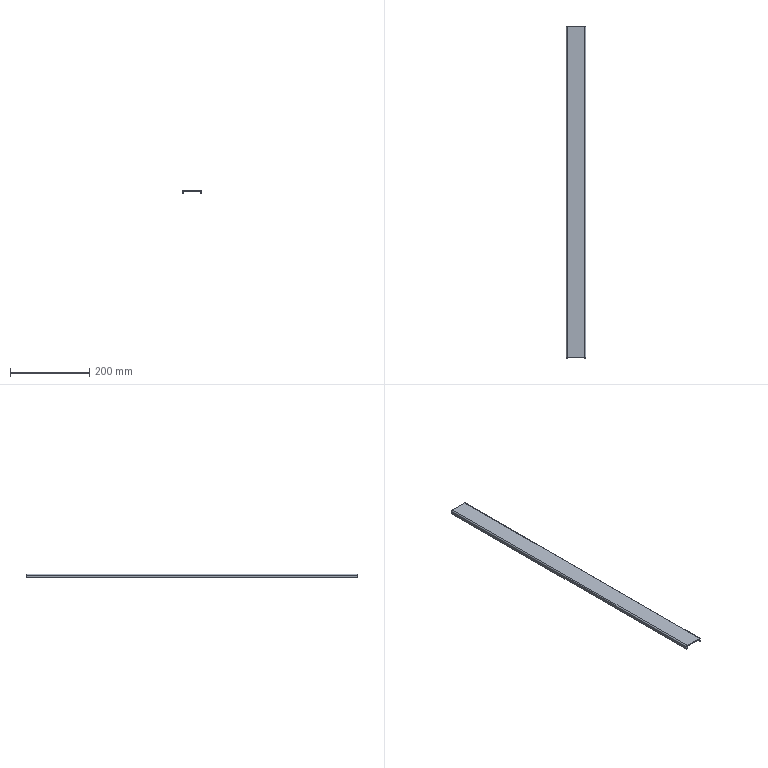Part | SolidWorks | features BaseBody 1 | 1 solid | 22 faces | box 50 x 839.8 x 10 mm | volume 133314 mm3 | plane 18 | cylinder 4 | commonest cylinder face diameters 1 x2 6 x2
STEP:
#1=CARTESIAN_POINT('',(-22.5,419.9,-10.));
#2=VERTEX_POINT('',#1);
#3=CARTESIAN_POINT('',(-22.5,-419.9,-10.));
#4=VERTEX_POINT('',#3);
#5=CARTESIAN_POINT('',(-22.5,-419.9,-10.));
#6=DIRECTION('',(0.,-1.,0.));
#7=VECTOR('',#6,1000.);
#8=LINE('',#5,#7);
#9=EDGE_CURVE('',#2,#4,#8,.T.);
#10=ORIENTED_EDGE('',*,*,#9,.T.);
#11=CARTESIAN_POINT('',(-25.,-419.9,-10.));
#12=VERTEX_POINT('',#11);
#13=CARTESIAN_POINT('',(-25.,-419.9,-10.));
#14=DIRECTION('',(1.,0.,0.));
#15=VECTOR('',#14,1000.);
#16=LINE('',#13,#15);
#17=EDGE_CURVE('',#12,#4,#16,.T.);
#18=ORIENTED_EDGE('',*,*,#17,.F.);
#19=CARTESIAN_POINT('',(-25.,419.9,-10.));
#20=VERTEX_POINT('',#19);
#21=CARTESIAN_POINT('',(-25.,0.,-10.));
#22=DIRECTION('',(0.,-1.,0.));
#23=VECTOR('',#22,1000.);
#24=LINE('',#21,#23);
#25=EDGE_CURVE('',#20,#12,#24,.T.);
#26=ORIENTED_EDGE('',*,*,#25,.F.);
#27=CARTESIAN_POINT('',(-25.,419.9,-10.));
#28=DIRECTION('',(1.,0.,0.));
#29=VECTOR('',#28,1000.);
#30=LINE('',#27,#29);
#31=EDGE_CURVE('',#20,#2,#30,.T.);
#32=ORIENTED_EDGE('',*,*,#31,.T.);
#33=EDGE_LOOP('',(#10,#18,#26,#32));
#34=FACE_OUTER_BOUND('',#33,.T.);
#35=CARTESIAN_POINT('',(-25.,-419.9,-10.));
#36=DIRECTION('',(0.,0.,1.));
#37=DIRECTION('',(1.,0.,0.));
#38=AXIS2_PLACEMENT_3D('',#35,#36,#37);
#39=PLANE('',#38);
#40=ADVANCED_FACE('',(#34),#39,.F.);
#41=CARTESIAN_POINT('',(-22.5,419.9,-3.));
#42=VERTEX_POINT('',#41);
#43=CARTESIAN_POINT('',(-22.5,419.9,-10.));
#44=DIRECTION('',(0.,0.,-1.));
#45=VECTOR('',#44,1000.);
#46=LINE('',#43,#45);
#47=EDGE_CURVE('',#42,#2,#46,.T.);
#48=ORIENTED_EDGE('',*,*,#47,.F.);
#49=CARTESIAN_POINT('',(-22.5,-419.9,-3.));
#50=VERTEX_POINT('',#49);
#51=CARTESIAN_POINT('',(-22.5,-419.9,-3.));
#52=DIRECTION('',(0.,1.,0.));
#53=VECTOR('',#52,1000.);
#54=LINE('',#51,#53);
#55=EDGE_CURVE('',#50,#42,#54,.T.);
#56=ORIENTED_EDGE('',*,*,#55,.F.);
#57=CARTESIAN_POINT('',(-22.5,-419.9,-2.5));
#58=DIRECTION('',(0.,0.,1.));
#59=VECTOR('',#58,1000.);
#60=LINE('',#57,#59);
#61=EDGE_CURVE('',#4,#50,#60,.T.);
#62=ORIENTED_EDGE('',*,*,#61,.F.);
#63=ORIENTED_EDGE('',*,*,#9,.F.);
#64=EDGE_LOOP('',(#48,#56,#62,#63));
#65=FACE_OUTER_BOUND('',#64,.T.);
#66=CARTESIAN_POINT('',(-22.5,0.,0.));
#67=DIRECTION('',(1.,0.,0.));
#68=DIRECTION('',(0.,0.,-1.));
#69=AXIS2_PLACEMENT_3D('',#66,#67,#68);
#70=PLANE('',#69);
#71=ADVANCED_FACE('',(#65),#70,.T.);
#72=CARTESIAN_POINT('',(-25.,419.9,-3.));
#73=VERTEX_POINT('',#72);
#74=CARTESIAN_POINT('',(-25.,-419.9,-3.));
#75=VERTEX_POINT('',#74);
#76=CARTESIAN_POINT('',(-25.,-419.9,-3.));
#77=DIRECTION('',(0.,-1.,0.));
#78=VECTOR('',#77,1000.);
#79=LINE('',#76,#78);
#80=EDGE_CURVE('',#73,#75,#79,.T.);
#81=ORIENTED_EDGE('',*,*,#80,.F.);
#82=CARTESIAN_POINT('',(-25.,419.9,0.));
#83=DIRECTION('',(0.,0.,-1.));
#84=VECTOR('',#83,1000.);
#85=LINE('',#82,#84);
#86=EDGE_CURVE('',#73,#20,#85,.T.);
#87=ORIENTED_EDGE('',*,*,#86,.T.);
#88=ORIENTED_EDGE('',*,*,#25,.T.);
#89=CARTESIAN_POINT('',(-25.,-419.9,0.));
#90=DIRECTION('',(0.,0.,1.));
#91=VECTOR('',#90,1000.);
#92=LINE('',#89,#91);
#93=EDGE_CURVE('',#12,#75,#92,.T.);
#94=ORIENTED_EDGE('',*,*,#93,.T.);
#95=EDGE_LOOP('',(#81,#87,#88,#94));
#96=FACE_OUTER_BOUND('',#95,.T.);
#97=CARTESIAN_POINT('',(-25.,0.,0.));
#98=DIRECTION('',(1.,0.,0.));
#99=DIRECTION('',(0.,0.,-1.));
#100=AXIS2_PLACEMENT_3D('',#97,#98,#99);
#101=PLANE('',#100);
#102=ADVANCED_FACE('',(#96),#101,.F.);
#103=CARTESIAN_POINT('',(-25.,-419.9,-3.));
#104=DIRECTION('',(-1.,0.,0.));
#105=VECTOR('',#104,1000.);
#106=LINE('',#103,#105);
#107=EDGE_CURVE('',#50,#75,#106,.T.);
#108=ORIENTED_EDGE('',*,*,#107,.T.);
#109=ORIENTED_EDGE('',*,*,#93,.F.);
#110=ORIENTED_EDGE('',*,*,#17,.T.);
#111=ORIENTED_EDGE('',*,*,#61,.T.);
#112=EDGE_LOOP('',(#108,#109,#110,#111));
#113=FACE_OUTER_BOUND('',#112,.T.);
#114=CARTESIAN_POINT('',(-25.,-419.9,-2.5));
#115=DIRECTION('',(0.,1.,0.));
#116=DIRECTION('',(0.,0.,-1.));
#117=AXIS2_PLACEMENT_3D('',#114,#115,#116);
#118=PLANE('',#117);
#119=ADVANCED_FACE('',(#113),#118,.F.);
#120=CARTESIAN_POINT('',(-22.5,419.9,-3.));
#121=DIRECTION('',(-1.,0.,0.));
#122=VECTOR('',#121,1000.);
#123=LINE('',#120,#122);
#124=EDGE_CURVE('',#42,#73,#123,.T.);
#125=ORIENTED_EDGE('',*,*,#124,.F.);
#126=ORIENTED_EDGE('',*,*,#47,.T.);
#127=ORIENTED_EDGE('',*,*,#31,.F.);
#128=ORIENTED_EDGE('',*,*,#86,.F.);
#129=EDGE_LOOP('',(#125,#126,#127,#128));
#130=FACE_OUTER_BOUND('',#129,.T.);
#131=CARTESIAN_POINT('',(-25.,419.9,-10.));
#132=DIRECTION('',(0.,-1.,0.));
#133=DIRECTION('',(0.,0.,-1.));
#134=AXIS2_PLACEMENT_3D('',#131,#132,#133);
#135=PLANE('',#134);
#136=ADVANCED_FACE('',(#130),#135,.F.);
#137=CARTESIAN_POINT('',(-22.,419.9,-2.5));
#138=VERTEX_POINT('',#137);
#139=CARTESIAN_POINT('',(-22.,-419.9,-2.5));
#140=VERTEX_POINT('',#139);
#141=CARTESIAN_POINT('',(-22.,419.9,-2.5));
#142=DIRECTION('',(0.,-1.,0.));
#143=VECTOR('',#142,1000.);
#144=LINE('',#141,#143);
#145=EDGE_CURVE('',#138,#140,#144,.T.);
#146=ORIENTED_EDGE('',*,*,#145,.T.);
#147=CARTESIAN_POINT('',(-22.,-419.9,-3.));
#148=DIRECTION('',(0.,-1.,0.));
#149=DIRECTION('',(0.,0.,1.));
#150=AXIS2_PLACEMENT_3D('',#147,#148,#149);
#151=CIRCLE('',#150,0.5);
#152=EDGE_CURVE('',#140,#50,#151,.T.);
#153=ORIENTED_EDGE('',*,*,#152,.T.);
#154=ORIENTED_EDGE('',*,*,#55,.T.);
#155=CARTESIAN_POINT('',(-22.,419.9,-3.));
#156=DIRECTION('',(0.,1.,0.));
#157=DIRECTION('',(0.,0.,1.));
#158=AXIS2_PLACEMENT_3D('',#155,#156,#157);
#159=CIRCLE('',#158,0.5);
#160=EDGE_CURVE('',#42,#138,#159,.T.);
#161=ORIENTED_EDGE('',*,*,#160,.T.);
#162=EDGE_LOOP('',(#146,#153,#154,#161));
#163=FACE_OUTER_BOUND('',#162,.T.);
#164=CARTESIAN_POINT('',(-22.,419.9,-3.));
#165=DIRECTION('',(0.,1.,0.));
#166=DIRECTION('',(-1.,0.,0.));
#167=AXIS2_PLACEMENT_3D('',#164,#165,#166);
#168=CYLINDRICAL_SURFACE('',#167,0.5);
#169=ADVANCED_FACE('',(#163),#168,.F.);
#170=CARTESIAN_POINT('',(-22.,419.9,0.));
#171=VERTEX_POINT('',#170);
#172=CARTESIAN_POINT('',(-22.,-419.9,0.));
#173=VERTEX_POINT('',#172);
#174=CARTESIAN_POINT('',(-22.,419.9,0.));
#175=DIRECTION('',(0.,-1.,0.));
#176=VECTOR('',#175,1000.);
#177=LINE('',#174,#176);
#178=EDGE_CURVE('',#171,#173,#177,.T.);
#179=ORIENTED_EDGE('',*,*,#178,.F.);
#180=CARTESIAN_POINT('',(-22.,419.9,-3.));
#181=DIRECTION('',(0.,1.,0.));
#182=DIRECTION('',(0.,0.,1.));
#183=AXIS2_PLACEMENT_3D('',#180,#181,#182);
#184=CIRCLE('',#183,3.);
#185=EDGE_CURVE('',#73,#171,#184,.T.);
#186=ORIENTED_EDGE('',*,*,#185,.F.);
#187=ORIENTED_EDGE('',*,*,#80,.T.);
#188=CARTESIAN_POINT('',(-22.,-419.9,-3.));
#189=DIRECTION('',(0.,-1.,0.));
#190=DIRECTION('',(0.,0.,1.));
#191=AXIS2_PLACEMENT_3D('',#188,#189,#190);
#192=CIRCLE('',#191,3.);
#193=EDGE_CURVE('',#173,#75,#192,.T.);
#194=ORIENTED_EDGE('',*,*,#193,.F.);
#195=EDGE_LOOP('',(#179,#186,#187,#194));
#196=FACE_OUTER_BOUND('',#195,.T.);
#197=CARTESIAN_POINT('',(-22.,419.9,-3.));
#198=DIRECTION('',(0.,1.,0.));
#199=DIRECTION('',(-1.,0.,0.));
#200=AXIS2_PLACEMENT_3D('',#197,#198,#199);
#201=CYLINDRICAL_SURFACE('',#200,3.);
#202=ADVANCED_FACE('',(#196),#201,.T.);
#203=ORIENTED_EDGE('',*,*,#160,.F.);
#204=ORIENTED_EDGE('',*,*,#124,.T.);
#205=ORIENTED_EDGE('',*,*,#185,.T.);
#206=CARTESIAN_POINT('',(-22.,419.9,-2.5));
#207=DIRECTION('',(0.,0.,1.));
#208=VECTOR('',#207,1000.);
#209=LINE('',#206,#208);
#210=EDGE_CURVE('',#138,#171,#209,.T.);
#211=ORIENTED_EDGE('',*,*,#210,.F.);
#212=EDGE_LOOP('',(#203,#204,#205,#211));
#213=FACE_OUTER_BOUND('',#212,.T.);
#214=CARTESIAN_POINT('',(-22.,419.9,-3.));
#215=DIRECTION('',(0.,-1.,0.));
#216=DIRECTION('',(0.,0.,-1.));
#217=AXIS2_PLACEMENT_3D('',#214,#215,#216);
#218=PLANE('',#217);
#219=ADVANCED_FACE('',(#213),#218,.F.);
#220=ORIENTED_EDGE('',*,*,#107,.F.);
#221=ORIENTED_EDGE('',*,*,#152,.F.);
#222=CARTESIAN_POINT('',(-22.,-419.9,-2.5));
#223=DIRECTION('',(0.,0.,1.));
#224=VECTOR('',#223,1000.);
#225=LINE('',#222,#224);
#226=EDGE_CURVE('',#140,#173,#225,.T.);
#227=ORIENTED_EDGE('',*,*,#226,.T.);
#228=ORIENTED_EDGE('',*,*,#193,.T.);
#229=EDGE_LOOP('',(#220,#221,#227,#228));
#230=FACE_OUTER_BOUND('',#229,.T.);
#231=CARTESIAN_POINT('',(-22.,-419.9,-3.));
#232=DIRECTION('',(0.,-1.,0.));
#233=DIRECTION('',(0.,0.,-1.));
#234=AXIS2_PLACEMENT_3D('',#231,#232,#233);
#235=PLANE('',#234);
#236=ADVANCED_FACE('',(#230),#235,.T.);
#237=CARTESIAN_POINT('',(22.5,-419.9,-10.));
#238=VERTEX_POINT('',#237);
#239=CARTESIAN_POINT('',(22.5,419.9,-10.));
#240=VERTEX_POINT('',#239);
#241=CARTESIAN_POINT('',(22.5,419.9,-10.));
#242=DIRECTION('',(0.,1.,0.));
#243=VECTOR('',#242,1000.);
#244=LINE('',#241,#243);
#245=EDGE_CURVE('',#238,#240,#244,.T.);
#246=ORIENTED_EDGE('',*,*,#245,.T.);
#247=CARTESIAN_POINT('',(25.,419.9,-10.));
#248=VERTEX_POINT('',#247);
#249=CARTESIAN_POINT('',(25.,419.9,-10.));
#250=DIRECTION('',(-1.,0.,0.));
#251=VECTOR('',#250,1000.);
#252=LINE('',#249,#251);
#253=EDGE_CURVE('',#248,#240,#252,.T.);
#254=ORIENTED_EDGE('',*,*,#253,.F.);
#255=CARTESIAN_POINT('',(25.,-419.9,-10.));
#256=VERTEX_POINT('',#255);
#257=CARTESIAN_POINT('',(25.,0.,-10.));
#258=DIRECTION('',(0.,1.,0.));
#259=VECTOR('',#258,1000.);
#260=LINE('',#257,#259);
#261=EDGE_CURVE('',#256,#248,#260,.T.);
#262=ORIENTED_EDGE('',*,*,#261,.F.);
#263=CARTESIAN_POINT('',(25.,-419.9,-10.));
#264=DIRECTION('',(-1.,0.,0.));
#265=VECTOR('',#264,1000.);
#266=LINE('',#263,#265);
#267=EDGE_CURVE('',#256,#238,#266,.T.);
#268=ORIENTED_EDGE('',*,*,#267,.T.);
#269=EDGE_LOOP('',(#246,#254,#262,#268));
#270=FACE_OUTER_BOUND('',#269,.T.);
#271=CARTESIAN_POINT('',(25.,419.9,-10.));
#272=DIRECTION('',(0.,0.,1.));
#273=DIRECTION('',(1.,0.,0.));
#274=AXIS2_PLACEMENT_3D('',#271,#272,#273);
#275=PLANE('',#274);
#276=ADVANCED_FACE('',(#270),#275,.F.);
#277=CARTESIAN_POINT('',(22.5,-419.9,-3.));
#278=VERTEX_POINT('',#277);
#279=CARTESIAN_POINT('',(22.5,-419.9,-10.));
#280=DIRECTION('',(0.,0.,-1.));
#281=VECTOR('',#280,1000.);
#282=LINE('',#279,#281);
#283=EDGE_CURVE('',#278,#238,#282,.T.);
#284=ORIENTED_EDGE('',*,*,#283,.F.);
#285=CARTESIAN_POINT('',(22.5,419.9,-3.));
#286=VERTEX_POINT('',#285);
#287=CARTESIAN_POINT('',(22.5,419.9,-3.));
#288=DIRECTION('',(0.,-1.,0.));
#289=VECTOR('',#288,1000.);
#290=LINE('',#287,#289);
#291=EDGE_CURVE('',#286,#278,#290,.T.);
#292=ORIENTED_EDGE('',*,*,#291,.F.);
#293=CARTESIAN_POINT('',(22.5,419.9,-2.5));
#294=DIRECTION('',(0.,0.,1.));
#295=VECTOR('',#294,1000.);
#296=LINE('',#293,#295);
#297=EDGE_CURVE('',#240,#286,#296,.T.);
#298=ORIENTED_EDGE('',*,*,#297,.F.);
#299=ORIENTED_EDGE('',*,*,#245,.F.);
#300=EDGE_LOOP('',(#284,#292,#298,#299));
#301=FACE_OUTER_BOUND('',#300,.T.);
#302=CARTESIAN_POINT('',(22.5,0.,0.));
#303=DIRECTION('',(-1.,0.,0.));
#304=DIRECTION('',(0.,0.,1.));
#305=AXIS2_PLACEMENT_3D('',#302,#303,#304);
#306=PLANE('',#305);
#307=ADVANCED_FACE('',(#301),#306,.T.);
#308=CARTESIAN_POINT('',(25.,-419.9,-3.));
#309=VERTEX_POINT('',#308);
#310=CARTESIAN_POINT('',(25.,419.9,-3.));
#311=VERTEX_POINT('',#310);
#312=CARTESIAN_POINT('',(25.,419.9,-3.));
#313=DIRECTION('',(0.,1.,0.));
#314=VECTOR('',#313,1000.);
#315=LINE('',#312,#314);
#316=EDGE_CURVE('',#309,#311,#315,.T.);
#317=ORIENTED_EDGE('',*,*,#316,.F.);
#318=CARTESIAN_POINT('',(25.,-419.9,0.));
#319=DIRECTION('',(0.,0.,-1.));
#320=VECTOR('',#319,1000.);
#321=LINE('',#318,#320);
#322=EDGE_CURVE('',#309,#256,#321,.T.);
#323=ORIENTED_EDGE('',*,*,#322,.T.);
#324=ORIENTED_EDGE('',*,*,#261,.T.);
#325=CARTESIAN_POINT('',(25.,419.9,0.));
#326=DIRECTION('',(0.,0.,1.));
#327=VECTOR('',#326,1000.);
#328=LINE('',#325,#327);
#329=EDGE_CURVE('',#248,#311,#328,.T.);
#330=ORIENTED_EDGE('',*,*,#329,.T.);
#331=EDGE_LOOP('',(#317,#323,#324,#330));
#332=FACE_OUTER_BOUND('',#331,.T.);
#333=CARTESIAN_POINT('',(25.,0.,0.));
#334=DIRECTION('',(-1.,0.,0.));
#335=DIRECTION('',(0.,0.,1.));
#336=AXIS2_PLACEMENT_3D('',#333,#334,#335);
#337=PLANE('',#336);
#338=ADVANCED_FACE('',(#332),#337,.F.);
#339=CARTESIAN_POINT('',(25.,419.9,-3.));
#340=DIRECTION('',(1.,0.,0.));
#341=VECTOR('',#340,1000.);
#342=LINE('',#339,#341);
#343=EDGE_CURVE('',#286,#311,#342,.T.);
#344=ORIENTED_EDGE('',*,*,#343,.T.);
#345=ORIENTED_EDGE('',*,*,#329,.F.);
#346=ORIENTED_EDGE('',*,*,#253,.T.);
#347=ORIENTED_EDGE('',*,*,#297,.T.);
#348=EDGE_LOOP('',(#344,#345,#346,#347));
#349=FACE_OUTER_BOUND('',#348,.T.);
#350=CARTESIAN_POINT('',(25.,419.9,-2.5));
#351=DIRECTION('',(0.,-1.,0.));
#352=DIRECTION('',(0.,0.,-1.));
#353=AXIS2_PLACEMENT_3D('',#350,#351,#352);
#354=PLANE('',#353);
#355=ADVANCED_FACE('',(#349),#354,.F.);
#356=CARTESIAN_POINT('',(22.5,-419.9,-3.));
#357=DIRECTION('',(1.,0.,0.));
#358=VECTOR('',#357,1000.);
#359=LINE('',#356,#358);
#360=EDGE_CURVE('',#278,#309,#359,.T.);
#361=ORIENTED_EDGE('',*,*,#360,.F.);
#362=ORIENTED_EDGE('',*,*,#283,.T.);
#363=ORIENTED_EDGE('',*,*,#267,.F.);
#364=ORIENTED_EDGE('',*,*,#322,.F.);
#365=EDGE_LOOP('',(#361,#362,#363,#364));
#366=FACE_OUTER_BOUND('',#365,.T.);
#367=CARTESIAN_POINT('',(25.,-419.9,-10.));
#368=DIRECTION('',(0.,1.,0.));
#369=DIRECTION('',(0.,0.,-1.));
#370=AXIS2_PLACEMENT_3D('',#367,#368,#369);
#371=PLANE('',#370);
#372=ADVANCED_FACE('',(#366),#371,.F.);
#373=CARTESIAN_POINT('',(22.,-419.9,-2.5));
#374=VERTEX_POINT('',#373);
#375=CARTESIAN_POINT('',(22.,419.9,-2.5));
#376=VERTEX_POINT('',#375);
#377=CARTESIAN_POINT('',(22.,-419.9,-2.5));
#378=DIRECTION('',(0.,1.,0.));
#379=VECTOR('',#378,1000.);
#380=LINE('',#377,#379);
#381=EDGE_CURVE('',#374,#376,#380,.T.);
#382=ORIENTED_EDGE('',*,*,#381,.T.);
#383=CARTESIAN_POINT('',(22.,419.9,-3.));
#384=DIRECTION('',(0.,1.,0.));
#385=DIRECTION('',(0.,0.,-1.));
#386=AXIS2_PLACEMENT_3D('',#383,#384,#385);
#387=CIRCLE('',#386,0.5);
#388=EDGE_CURVE('',#376,#286,#387,.T.);
#389=ORIENTED_EDGE('',*,*,#388,.T.);
#390=ORIENTED_EDGE('',*,*,#291,.T.);
#391=CARTESIAN_POINT('',(22.,-419.9,-3.));
#392=DIRECTION('',(0.,-1.,0.));
#393=DIRECTION('',(0.,0.,-1.));
#394=AXIS2_PLACEMENT_3D('',#391,#392,#393);
#395=CIRCLE('',#394,0.5);
#396=EDGE_CURVE('',#278,#374,#395,.T.);
#397=ORIENTED_EDGE('',*,*,#396,.T.);
#398=EDGE_LOOP('',(#382,#389,#390,#397));
#399=FACE_OUTER_BOUND('',#398,.T.);
#400=CARTESIAN_POINT('',(22.,-419.9,-3.));
#401=DIRECTION('',(0.,-1.,0.));
#402=DIRECTION('',(1.,0.,0.));
#403=AXIS2_PLACEMENT_3D('',#400,#401,#402);
#404=CYLINDRICAL_SURFACE('',#403,0.5);
#405=ADVANCED_FACE('',(#399),#404,.F.);
#406=CARTESIAN_POINT('',(22.,-419.9,0.));
#407=VERTEX_POINT('',#406);
#408=CARTESIAN_POINT('',(22.,419.9,0.));
#409=VERTEX_POINT('',#408);
#410=CARTESIAN_POINT('',(22.,-419.9,0.));
#411=DIRECTION('',(0.,1.,0.));
#412=VECTOR('',#411,1000.);
#413=LINE('',#410,#412);
#414=EDGE_CURVE('',#407,#409,#413,.T.);
#415=ORIENTED_EDGE('',*,*,#414,.F.);
#416=CARTESIAN_POINT('',(22.,-419.9,-3.));
#417=DIRECTION('',(0.,-1.,0.));
#418=DIRECTION('',(0.,0.,-1.));
#419=AXIS2_PLACEMENT_3D('',#416,#417,#418);
#420=CIRCLE('',#419,3.);
#421=EDGE_CURVE('',#309,#407,#420,.T.);
#422=ORIENTED_EDGE('',*,*,#421,.F.);
#423=ORIENTED_EDGE('',*,*,#316,.T.);
#424=CARTESIAN_POINT('',(22.,419.9,-3.));
#425=DIRECTION('',(0.,1.,0.));
#426=DIRECTION('',(0.,0.,-1.));
#427=AXIS2_PLACEMENT_3D('',#424,#425,#426);
#428=CIRCLE('',#427,3.);
#429=EDGE_CURVE('',#409,#311,#428,.T.);
#430=ORIENTED_EDGE('',*,*,#429,.F.);
#431=EDGE_LOOP('',(#415,#422,#423,#430));
#432=FACE_OUTER_BOUND('',#431,.T.);
#433=CARTESIAN_POINT('',(22.,-419.9,-3.));
#434=DIRECTION('',(0.,-1.,0.));
#435=DIRECTION('',(1.,0.,0.));
#436=AXIS2_PLACEMENT_3D('',#433,#434,#435);
#437=CYLINDRICAL_SURFACE('',#436,3.);
#438=ADVANCED_FACE('',(#432),#437,.T.);
#439=ORIENTED_EDGE('',*,*,#396,.F.);
#440=ORIENTED_EDGE('',*,*,#360,.T.);
#441=ORIENTED_EDGE('',*,*,#421,.T.);
#442=CARTESIAN_POINT('',(22.,-419.9,-2.5));
#443=DIRECTION('',(0.,0.,1.));
#444=VECTOR('',#443,1000.);
#445=LINE('',#442,#444);
#446=EDGE_CURVE('',#374,#407,#445,.T.);
#447=ORIENTED_EDGE('',*,*,#446,.F.);
#448=EDGE_LOOP('',(#439,#440,#441,#447));
#449=FACE_OUTER_BOUND('',#448,.T.);
#450=CARTESIAN_POINT('',(22.,-419.9,-3.));
#451=DIRECTION('',(0.,1.,0.));
#452=DIRECTION('',(1.,0.,0.));
#453=AXIS2_PLACEMENT_3D('',#450,#451,#452);
#454=PLANE('',#453);
#455=ADVANCED_FACE('',(#449),#454,.F.);
#456=ORIENTED_EDGE('',*,*,#343,.F.);
#457=ORIENTED_EDGE('',*,*,#388,.F.);
#458=CARTESIAN_POINT('',(22.,419.9,-2.5));
#459=DIRECTION('',(0.,0.,1.));
#460=VECTOR('',#459,1000.);
#461=LINE('',#458,#460);
#462=EDGE_CURVE('',#376,#409,#461,.T.);
#463=ORIENTED_EDGE('',*,*,#462,.T.);
#464=ORIENTED_EDGE('',*,*,#429,.T.);
#465=EDGE_LOOP('',(#456,#457,#463,#464));
#466=FACE_OUTER_BOUND('',#465,.T.);
#467=CARTESIAN_POINT('',(22.,419.9,-3.));
#468=DIRECTION('',(0.,1.,0.));
#469=DIRECTION('',(1.,0.,0.));
#470=AXIS2_PLACEMENT_3D('',#467,#468,#469);
#471=PLANE('',#470);
#472=ADVANCED_FACE('',(#466),#471,.T.);
#473=ORIENTED_EDGE('',*,*,#226,.F.);
#474=CARTESIAN_POINT('',(25.,-419.9,-2.5));
#475=DIRECTION('',(1.,0.,0.));
#476=VECTOR('',#475,1000.);
#477=LINE('',#474,#476);
#478=EDGE_CURVE('',#140,#374,#477,.T.);
#479=ORIENTED_EDGE('',*,*,#478,.T.);
#480=ORIENTED_EDGE('',*,*,#446,.T.);
#481=CARTESIAN_POINT('',(25.,-419.9,0.));
#482=DIRECTION('',(1.,0.,0.));
#483=VECTOR('',#482,1000.);
#484=LINE('',#481,#483);
#485=EDGE_CURVE('',#173,#407,#484,.T.);
#486=ORIENTED_EDGE('',*,*,#485,.F.);
#487=EDGE_LOOP('',(#473,#479,#480,#486));
#488=FACE_OUTER_BOUND('',#487,.T.);
#489=CARTESIAN_POINT('',(25.,-419.9,-2.5));
#490=DIRECTION('',(0.,-1.,0.));
#491=DIRECTION('',(0.,0.,-1.));
#492=AXIS2_PLACEMENT_3D('',#489,#490,#491);
#493=PLANE('',#492);
#494=ADVANCED_FACE('',(#488),#493,.T.);
#495=CARTESIAN_POINT('',(25.,419.9,-2.5));
#496=DIRECTION('',(-1.,0.,0.));
#497=VECTOR('',#496,1000.);
#498=LINE('',#495,#497);
#499=EDGE_CURVE('',#376,#138,#498,.T.);
#500=ORIENTED_EDGE('',*,*,#499,.T.);
#501=ORIENTED_EDGE('',*,*,#210,.T.);
#502=CARTESIAN_POINT('',(25.,419.9,0.));
#503=DIRECTION('',(-1.,0.,0.));
#504=VECTOR('',#503,1000.);
#505=LINE('',#502,#504);
#506=EDGE_CURVE('',#409,#171,#505,.T.);
#507=ORIENTED_EDGE('',*,*,#506,.F.);
#508=ORIENTED_EDGE('',*,*,#462,.F.);
#509=EDGE_LOOP('',(#500,#501,#507,#508));
#510=FACE_OUTER_BOUND('',#509,.T.);
#511=CARTESIAN_POINT('',(25.,419.9,-2.5));
#512=DIRECTION('',(0.,1.,0.));
#513=DIRECTION('',(1.,0.,0.));
#514=AXIS2_PLACEMENT_3D('',#511,#512,#513);
#515=PLANE('',#514);
#516=ADVANCED_FACE('',(#510),#515,.T.);
#517=ORIENTED_EDGE('',*,*,#178,.T.);
#518=ORIENTED_EDGE('',*,*,#485,.T.);
#519=ORIENTED_EDGE('',*,*,#414,.T.);
#520=ORIENTED_EDGE('',*,*,#506,.T.);
#521=EDGE_LOOP('',(#517,#518,#519,#520));
#522=FACE_OUTER_BOUND('',#521,.T.);
#523=CARTESIAN_POINT('',(0.,0.,0.));
#524=DIRECTION('',(0.,0.,-1.));
#525=DIRECTION('',(0.,-1.,0.));
#526=AXIS2_PLACEMENT_3D('',#523,#524,#525);
#527=PLANE('',#526);
#528=ADVANCED_FACE('',(#522),#527,.F.);
#529=ORIENTED_EDGE('',*,*,#478,.F.);
#530=ORIENTED_EDGE('',*,*,#145,.F.);
#531=ORIENTED_EDGE('',*,*,#499,.F.);
#532=ORIENTED_EDGE('',*,*,#381,.F.);
#533=EDGE_LOOP('',(#529,#530,#531,#532));
#534=FACE_OUTER_BOUND('',#533,.T.);
#535=CARTESIAN_POINT('',(0.,0.,-2.5));
#536=DIRECTION('',(0.,0.,-1.));
#537=DIRECTION('',(0.,-1.,0.));
#538=AXIS2_PLACEMENT_3D('',#535,#536,#537);
#539=PLANE('',#538);
#540=ADVANCED_FACE('',(#534),#539,.T.);
#541=CLOSED_SHELL('',(#40,#71,#102,#119,#136,#169,#202,#219,#236,#276,#307,#338,#355,#372,#405,#438,#455,#472,#494,#516,#528,#540));
#542=MANIFOLD_SOLID_BREP('',#541);
#543=CARTESIAN_POINT('',(0.,0.,0.));
#544=DIRECTION('',(0.,0.,1.));
#545=DIRECTION('',(1.,0.,0.));
#546=AXIS2_PLACEMENT_3D('',#543,#544,#545);
#547=(LENGTH_UNIT()NAMED_UNIT(*)SI_UNIT(.MILLI.,.METRE.));
#548=UNCERTAINTY_MEASURE_WITH_UNIT(LENGTH_MEASURE(0.00001),#547,'','');
#549=(NAMED_UNIT(*)PLANE_ANGLE_UNIT()SI_UNIT($,.RADIAN.));
#550=(NAMED_UNIT(*)SI_UNIT($,.STERADIAN.)SOLID_ANGLE_UNIT());
#551=(GEOMETRIC_REPRESENTATION_CONTEXT(3)GLOBAL_UNCERTAINTY_ASSIGNED_CONTEXT((#548))GLOBAL_UNIT_ASSIGNED_CONTEXT((#547,#549,#550))REPRESENTATION_CONTEXT('',''));
#552=ADVANCED_BREP_SHAPE_REPRESENTATION('',(#542,#546),#551);